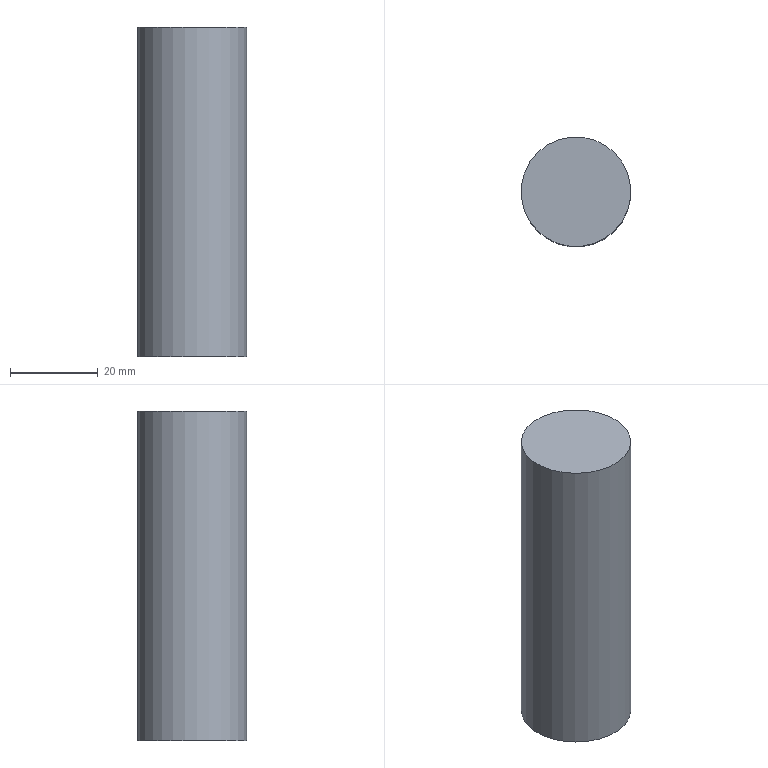Part | NX | features solid 2 | 1 solid | 3 faces | box 25 x 25 x 75 mm | volume 36816 mm3 | plane 2 | cylinder 1 | commonest cylinder face diameters 25 x1
STEP:
#1=CARTESIAN_POINT('',(1283.254,-245.725,268.));
#2=VERTEX_POINT('',#1);
#3=CARTESIAN_POINT('',(1295.,-250.,268.));
#4=DIRECTION('',(0.,0.,-1.));
#5=DIRECTION('',(-0.9397,0.342,0.));
#6=AXIS2_PLACEMENT_3D('',#3,#4,#5);
#7=CIRCLE('',#6,12.5);
#8=EDGE_CURVE('',#2,#2,#7,.T.);
#9=ORIENTED_EDGE('',*,*,#8,.T.);
#10=EDGE_LOOP('',(#9));
#11=FACE_BOUND('',#10,.T.);
#12=CARTESIAN_POINT('',(1283.254,-245.725,193.));
#13=VERTEX_POINT('',#12);
#14=CARTESIAN_POINT('',(1295.,-250.,193.));
#15=DIRECTION('',(0.,0.,-1.));
#16=DIRECTION('',(-0.9397,0.342,0.));
#17=AXIS2_PLACEMENT_3D('',#14,#15,#16);
#18=CIRCLE('',#17,12.5);
#19=EDGE_CURVE('',#13,#13,#18,.T.);
#20=ORIENTED_EDGE('',*,*,#19,.F.);
#21=EDGE_LOOP('',(#20));
#22=FACE_BOUND('',#21,.T.);
#23=CARTESIAN_POINT('',(1295.,-250.,268.));
#24=DIRECTION('',(0.,0.,-1.));
#25=DIRECTION('',(-0.9397,0.342,0.));
#26=AXIS2_PLACEMENT_3D('',#23,#24,#25);
#27=CYLINDRICAL_SURFACE('',#26,12.5);
#28=ADVANCED_FACE('',(#11,#22),#27,.T.);
#29=ORIENTED_EDGE('',*,*,#8,.F.);
#30=EDGE_LOOP('',(#29));
#31=FACE_BOUND('',#30,.T.);
#32=CARTESIAN_POINT('',(1295.,-250.,268.));
#33=DIRECTION('',(0.,0.,-1.));
#34=DIRECTION('',(-0.9397,0.342,0.));
#35=AXIS2_PLACEMENT_3D('',#32,#33,#34);
#36=PLANE('',#35);
#37=ADVANCED_FACE('',(#31),#36,.F.);
#38=ORIENTED_EDGE('',*,*,#19,.T.);
#39=EDGE_LOOP('',(#38));
#40=FACE_BOUND('',#39,.T.);
#41=CARTESIAN_POINT('',(1295.,-250.,193.));
#42=DIRECTION('',(0.,0.,-1.));
#43=DIRECTION('',(-0.9397,0.342,0.));
#44=AXIS2_PLACEMENT_3D('',#41,#42,#43);
#45=PLANE('',#44);
#46=ADVANCED_FACE('',(#40),#45,.T.);
#47=CLOSED_SHELL('',(#28,#37,#46));
#48=MANIFOLD_SOLID_BREP('',#47);
#49=(LENGTH_UNIT()NAMED_UNIT(*)SI_UNIT(.MILLI.,.METRE.));
#50=UNCERTAINTY_MEASURE_WITH_UNIT(LENGTH_MEASURE(0.00001),#49,'','');
#51=(NAMED_UNIT(*)PLANE_ANGLE_UNIT()SI_UNIT($,.RADIAN.));
#52=(NAMED_UNIT(*)SI_UNIT($,.STERADIAN.)SOLID_ANGLE_UNIT());
#53=(GEOMETRIC_REPRESENTATION_CONTEXT(3)GLOBAL_UNCERTAINTY_ASSIGNED_CONTEXT((#50))GLOBAL_UNIT_ASSIGNED_CONTEXT((#49,#51,#52))REPRESENTATION_CONTEXT('',''));
#54=ADVANCED_BREP_SHAPE_REPRESENTATION('',(#48),#53);